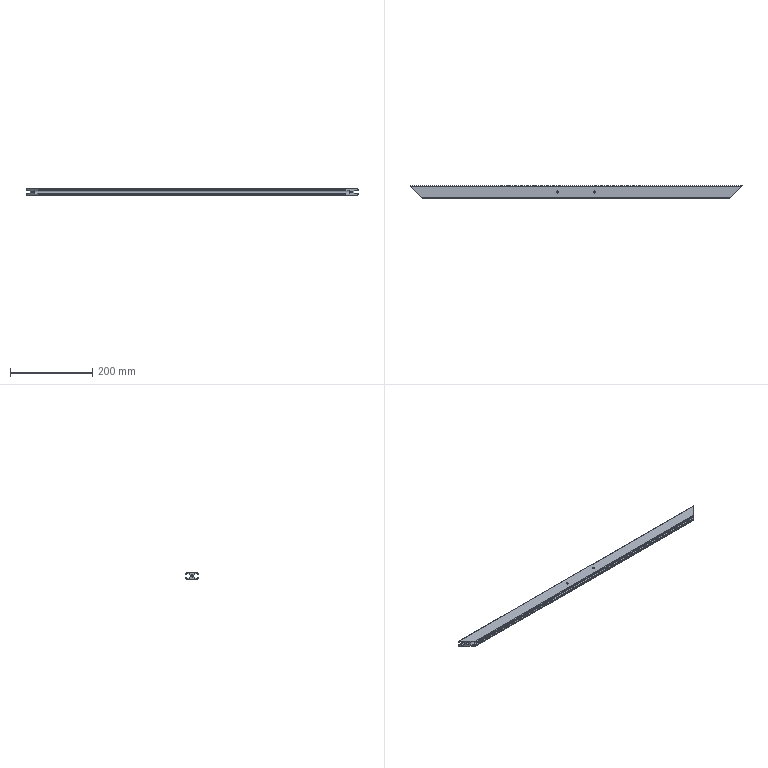Part | SolidWorks | features 3DProfileFeature 1, HoleWzd 1, ICE 1, WeldMemberFeat 1, WeldmentFeature 1 | 1 solid | 40 faces | box 805 x 30 x 15 mm | volume 190827 mm3 | cylinder 20 | plane 20 | commonest cylinder face diameters 5 x14 3 x4 12 x2
STEP:
#1=CARTESIAN_POINT('',(-45.,-2.5,0.));
#2=VERTEX_POINT('',#1);
#3=CARTESIAN_POINT('',(-47.5,0.,2.5));
#4=VERTEX_POINT('',#3);
#5=CARTESIAN_POINT('',(-45.,-2.5,0.));
#6=CARTESIAN_POINT('',(-46.464,-2.5,1.464));
#7=CARTESIAN_POINT('',(-47.5,-1.464,2.5));
#8=CARTESIAN_POINT('',(-47.5,0.,2.5));
#9=(BOUNDED_CURVE()B_SPLINE_CURVE(3,(#5,#6,#7,#8),.UNSPECIFIED.,.F.,.F.)B_SPLINE_CURVE_WITH_KNOTS((4,4),(4.712,6.283),.UNSPECIFIED.)CURVE()GEOMETRIC_REPRESENTATION_ITEM()RATIONAL_B_SPLINE_CURVE((1.,0.8047,0.8047,1.))REPRESENTATION_ITEM(''));
#10=EDGE_CURVE('',#2,#4,#9,.T.);
#11=ORIENTED_EDGE('',*,*,#10,.T.);
#12=CARTESIAN_POINT('',(-47.5,0.,7.5));
#13=VERTEX_POINT('',#12);
#14=CARTESIAN_POINT('',(-47.5,0.,7.5));
#15=DIRECTION('',(0.,0.,1.));
#16=VECTOR('',#15,1000.);
#17=LINE('',#14,#16);
#18=EDGE_CURVE('',#4,#13,#17,.T.);
#19=ORIENTED_EDGE('',*,*,#18,.T.);
#20=CARTESIAN_POINT('',(-42.5,0.,7.5));
#21=VERTEX_POINT('',#20);
#22=CARTESIAN_POINT('',(-45.,0.,7.5));
#23=DIRECTION('',(0.,0.,1.));
#24=DIRECTION('',(1.,0.,0.));
#25=AXIS2_PLACEMENT_3D('',#22,#23,#24);
#26=CIRCLE('',#25,2.5);
#27=EDGE_CURVE('',#13,#21,#26,.T.);
#28=ORIENTED_EDGE('',*,*,#27,.T.);
#29=CARTESIAN_POINT('',(-42.5,0.,2.5));
#30=VERTEX_POINT('',#29);
#31=CARTESIAN_POINT('',(-42.5,0.,7.5));
#32=DIRECTION('',(0.,0.,1.));
#33=VECTOR('',#32,1000.);
#34=LINE('',#31,#33);
#35=EDGE_CURVE('',#30,#21,#34,.T.);
#36=ORIENTED_EDGE('',*,*,#35,.F.);
#37=CARTESIAN_POINT('',(-42.5,0.,2.5));
#38=CARTESIAN_POINT('',(-42.5,-1.464,2.5));
#39=CARTESIAN_POINT('',(-43.536,-2.5,1.464));
#40=CARTESIAN_POINT('',(-45.,-2.5,0.));
#41=(BOUNDED_CURVE()B_SPLINE_CURVE(3,(#37,#38,#39,#40),.UNSPECIFIED.,.F.,.F.)B_SPLINE_CURVE_WITH_KNOTS((4,4),(3.142,4.712),.UNSPECIFIED.)CURVE()GEOMETRIC_REPRESENTATION_ITEM()RATIONAL_B_SPLINE_CURVE((1.,0.8047,0.8047,1.))REPRESENTATION_ITEM(''));
#42=EDGE_CURVE('',#30,#2,#41,.T.);
#43=ORIENTED_EDGE('',*,*,#42,.T.);
#44=EDGE_LOOP('',(#11,#19,#28,#36,#43));
#45=FACE_OUTER_BOUND('',#44,.T.);
#46=CARTESIAN_POINT('',(-45.,0.,7.5));
#47=DIRECTION('',(0.,0.,1.));
#48=DIRECTION('',(1.,0.,0.));
#49=AXIS2_PLACEMENT_3D('',#46,#47,#48);
#50=CYLINDRICAL_SURFACE('',#49,2.5);
#51=ADVANCED_FACE('',(#45),#50,.F.);
#52=CARTESIAN_POINT('',(-47.5,0.,-7.5));
#53=VERTEX_POINT('',#52);
#54=CARTESIAN_POINT('',(-42.5,0.,-7.5));
#55=VERTEX_POINT('',#54);
#56=CARTESIAN_POINT('',(-45.,0.,-7.5));
#57=DIRECTION('',(0.,0.,1.));
#58=DIRECTION('',(1.,0.,0.));
#59=AXIS2_PLACEMENT_3D('',#56,#57,#58);
#60=CIRCLE('',#59,2.5);
#61=EDGE_CURVE('',#53,#55,#60,.T.);
#62=ORIENTED_EDGE('',*,*,#61,.F.);
#63=CARTESIAN_POINT('',(-47.5,0.,-2.5));
#64=VERTEX_POINT('',#63);
#65=CARTESIAN_POINT('',(-47.5,0.,7.5));
#66=DIRECTION('',(0.,0.,1.));
#67=VECTOR('',#66,1000.);
#68=LINE('',#65,#67);
#69=EDGE_CURVE('',#53,#64,#68,.T.);
#70=ORIENTED_EDGE('',*,*,#69,.T.);
#71=CARTESIAN_POINT('',(-47.5,0.,-2.5));
#72=CARTESIAN_POINT('',(-47.5,-1.464,-2.5));
#73=CARTESIAN_POINT('',(-46.464,-2.5,-1.464));
#74=CARTESIAN_POINT('',(-45.,-2.5,0.));
#75=(BOUNDED_CURVE()B_SPLINE_CURVE(3,(#71,#72,#73,#74),.UNSPECIFIED.,.F.,.F.)B_SPLINE_CURVE_WITH_KNOTS((4,4),(0.,1.571),.UNSPECIFIED.)CURVE()GEOMETRIC_REPRESENTATION_ITEM()RATIONAL_B_SPLINE_CURVE((1.,0.8047,0.8047,1.))REPRESENTATION_ITEM(''));
#76=EDGE_CURVE('',#64,#2,#75,.T.);
#77=ORIENTED_EDGE('',*,*,#76,.T.);
#78=CARTESIAN_POINT('',(-42.5,0.,-2.5));
#79=VERTEX_POINT('',#78);
#80=CARTESIAN_POINT('',(-45.,-2.5,0.));
#81=CARTESIAN_POINT('',(-43.536,-2.5,-1.464));
#82=CARTESIAN_POINT('',(-42.5,-1.464,-2.5));
#83=CARTESIAN_POINT('',(-42.5,0.,-2.5));
#84=(BOUNDED_CURVE()B_SPLINE_CURVE(3,(#80,#81,#82,#83),.UNSPECIFIED.,.F.,.F.)B_SPLINE_CURVE_WITH_KNOTS((4,4),(1.571,3.142),.UNSPECIFIED.)CURVE()GEOMETRIC_REPRESENTATION_ITEM()RATIONAL_B_SPLINE_CURVE((1.,0.8047,0.8047,1.))REPRESENTATION_ITEM(''));
#85=EDGE_CURVE('',#2,#79,#84,.T.);
#86=ORIENTED_EDGE('',*,*,#85,.T.);
#87=CARTESIAN_POINT('',(-42.5,0.,7.5));
#88=DIRECTION('',(0.,0.,1.));
#89=VECTOR('',#88,1000.);
#90=LINE('',#87,#89);
#91=EDGE_CURVE('',#55,#79,#90,.T.);
#92=ORIENTED_EDGE('',*,*,#91,.F.);
#93=EDGE_LOOP('',(#62,#70,#77,#86,#92));
#94=FACE_OUTER_BOUND('',#93,.T.);
#95=CARTESIAN_POINT('',(-45.,0.,7.5));
#96=DIRECTION('',(0.,0.,1.));
#97=DIRECTION('',(1.,0.,0.));
#98=AXIS2_PLACEMENT_3D('',#95,#96,#97);
#99=CYLINDRICAL_SURFACE('',#98,2.5);
#100=ADVANCED_FACE('',(#94),#99,.F.);
#101=CARTESIAN_POINT('',(45.,-2.5,0.));
#102=VERTEX_POINT('',#101);
#103=CARTESIAN_POINT('',(42.5,0.,2.5));
#104=VERTEX_POINT('',#103);
#105=CARTESIAN_POINT('',(45.,-2.5,0.));
#106=CARTESIAN_POINT('',(43.536,-2.5,1.464));
#107=CARTESIAN_POINT('',(42.5,-1.464,2.5));
#108=CARTESIAN_POINT('',(42.5,0.,2.5));
#109=(BOUNDED_CURVE()B_SPLINE_CURVE(3,(#105,#106,#107,#108),.UNSPECIFIED.,.F.,.F.)B_SPLINE_CURVE_WITH_KNOTS((4,4),(4.712,6.283),.UNSPECIFIED.)CURVE()GEOMETRIC_REPRESENTATION_ITEM()RATIONAL_B_SPLINE_CURVE((1.,0.8047,0.8047,1.))REPRESENTATION_ITEM(''));
#110=EDGE_CURVE('',#102,#104,#109,.T.);
#111=ORIENTED_EDGE('',*,*,#110,.T.);
#112=CARTESIAN_POINT('',(42.5,0.,7.5));
#113=VERTEX_POINT('',#112);
#114=CARTESIAN_POINT('',(42.5,0.,7.5));
#115=DIRECTION('',(0.,0.,1.));
#116=VECTOR('',#115,1000.);
#117=LINE('',#114,#116);
#118=EDGE_CURVE('',#104,#113,#117,.T.);
#119=ORIENTED_EDGE('',*,*,#118,.T.);
#120=CARTESIAN_POINT('',(47.5,0.,7.5));
#121=VERTEX_POINT('',#120);
#122=CARTESIAN_POINT('',(45.,0.,7.5));
#123=DIRECTION('',(0.,0.,1.));
#124=DIRECTION('',(1.,0.,0.));
#125=AXIS2_PLACEMENT_3D('',#122,#123,#124);
#126=CIRCLE('',#125,2.5);
#127=EDGE_CURVE('',#113,#121,#126,.T.);
#128=ORIENTED_EDGE('',*,*,#127,.T.);
#129=CARTESIAN_POINT('',(47.5,0.,2.5));
#130=VERTEX_POINT('',#129);
#131=CARTESIAN_POINT('',(47.5,0.,7.5));
#132=DIRECTION('',(0.,0.,1.));
#133=VECTOR('',#132,1000.);
#134=LINE('',#131,#133);
#135=EDGE_CURVE('',#130,#121,#134,.T.);
#136=ORIENTED_EDGE('',*,*,#135,.F.);
#137=CARTESIAN_POINT('',(47.5,0.,2.5));
#138=CARTESIAN_POINT('',(47.5,-1.464,2.5));
#139=CARTESIAN_POINT('',(46.464,-2.5,1.464));
#140=CARTESIAN_POINT('',(45.,-2.5,0.));
#141=(BOUNDED_CURVE()B_SPLINE_CURVE(3,(#137,#138,#139,#140),.UNSPECIFIED.,.F.,.F.)B_SPLINE_CURVE_WITH_KNOTS((4,4),(3.142,4.712),.UNSPECIFIED.)CURVE()GEOMETRIC_REPRESENTATION_ITEM()RATIONAL_B_SPLINE_CURVE((1.,0.8047,0.8047,1.))REPRESENTATION_ITEM(''));
#142=EDGE_CURVE('',#130,#102,#141,.T.);
#143=ORIENTED_EDGE('',*,*,#142,.T.);
#144=EDGE_LOOP('',(#111,#119,#128,#136,#143));
#145=FACE_OUTER_BOUND('',#144,.T.);
#146=CARTESIAN_POINT('',(45.,0.,7.5));
#147=DIRECTION('',(0.,0.,1.));
#148=DIRECTION('',(1.,0.,0.));
#149=AXIS2_PLACEMENT_3D('',#146,#147,#148);
#150=CYLINDRICAL_SURFACE('',#149,2.5);
#151=ADVANCED_FACE('',(#145),#150,.F.);
#152=CARTESIAN_POINT('',(42.5,0.,-7.5));
#153=VERTEX_POINT('',#152);
#154=CARTESIAN_POINT('',(47.5,0.,-7.5));
#155=VERTEX_POINT('',#154);
#156=CARTESIAN_POINT('',(45.,0.,-7.5));
#157=DIRECTION('',(0.,0.,1.));
#158=DIRECTION('',(1.,0.,0.));
#159=AXIS2_PLACEMENT_3D('',#156,#157,#158);
#160=CIRCLE('',#159,2.5);
#161=EDGE_CURVE('',#153,#155,#160,.T.);
#162=ORIENTED_EDGE('',*,*,#161,.F.);
#163=CARTESIAN_POINT('',(42.5,0.,-2.5));
#164=VERTEX_POINT('',#163);
#165=CARTESIAN_POINT('',(42.5,0.,7.5));
#166=DIRECTION('',(0.,0.,1.));
#167=VECTOR('',#166,1000.);
#168=LINE('',#165,#167);
#169=EDGE_CURVE('',#153,#164,#168,.T.);
#170=ORIENTED_EDGE('',*,*,#169,.T.);
#171=CARTESIAN_POINT('',(42.5,0.,-2.5));
#172=CARTESIAN_POINT('',(42.5,-1.464,-2.5));
#173=CARTESIAN_POINT('',(43.536,-2.5,-1.464));
#174=CARTESIAN_POINT('',(45.,-2.5,0.));
#175=(BOUNDED_CURVE()B_SPLINE_CURVE(3,(#171,#172,#173,#174),.UNSPECIFIED.,.F.,.F.)B_SPLINE_CURVE_WITH_KNOTS((4,4),(0.,1.571),.UNSPECIFIED.)CURVE()GEOMETRIC_REPRESENTATION_ITEM()RATIONAL_B_SPLINE_CURVE((1.,0.8047,0.8047,1.))REPRESENTATION_ITEM(''));
#176=EDGE_CURVE('',#164,#102,#175,.T.);
#177=ORIENTED_EDGE('',*,*,#176,.T.);
#178=CARTESIAN_POINT('',(47.5,0.,-2.5));
#179=VERTEX_POINT('',#178);
#180=CARTESIAN_POINT('',(45.,-2.5,0.));
#181=CARTESIAN_POINT('',(46.464,-2.5,-1.464));
#182=CARTESIAN_POINT('',(47.5,-1.464,-2.5));
#183=CARTESIAN_POINT('',(47.5,0.,-2.5));
#184=(BOUNDED_CURVE()B_SPLINE_CURVE(3,(#180,#181,#182,#183),.UNSPECIFIED.,.F.,.F.)B_SPLINE_CURVE_WITH_KNOTS((4,4),(1.571,3.142),.UNSPECIFIED.)CURVE()GEOMETRIC_REPRESENTATION_ITEM()RATIONAL_B_SPLINE_CURVE((1.,0.8047,0.8047,1.))REPRESENTATION_ITEM(''));
#185=EDGE_CURVE('',#102,#179,#184,.T.);
#186=ORIENTED_EDGE('',*,*,#185,.T.);
#187=CARTESIAN_POINT('',(47.5,0.,7.5));
#188=DIRECTION('',(0.,0.,1.));
#189=VECTOR('',#188,1000.);
#190=LINE('',#187,#189);
#191=EDGE_CURVE('',#155,#179,#190,.T.);
#192=ORIENTED_EDGE('',*,*,#191,.F.);
#193=EDGE_LOOP('',(#162,#170,#177,#186,#192));
#194=FACE_OUTER_BOUND('',#193,.T.);
#195=CARTESIAN_POINT('',(45.,0.,7.5));
#196=DIRECTION('',(0.,0.,1.));
#197=DIRECTION('',(1.,0.,0.));
#198=AXIS2_PLACEMENT_3D('',#195,#196,#197);
#199=CYLINDRICAL_SURFACE('',#198,2.5);
#200=ADVANCED_FACE('',(#194),#199,.F.);
#201=ORIENTED_EDGE('',*,*,#76,.F.);
#202=CARTESIAN_POINT('',(-387.5,0.,-2.5));
#203=VERTEX_POINT('',#202);
#204=CARTESIAN_POINT('',(402.5,0.,-2.5));
#205=DIRECTION('',(-1.,0.,0.));
#206=VECTOR('',#205,1000.);
#207=LINE('',#204,#206);
#208=EDGE_CURVE('',#64,#203,#207,.T.);
#209=ORIENTED_EDGE('',*,*,#208,.T.);
#210=CARTESIAN_POINT('',(-387.5,0.,2.5));
#211=VERTEX_POINT('',#210);
#212=CARTESIAN_POINT('',(-387.5,0.,2.5));
#213=CARTESIAN_POINT('',(-382.5,-5.,2.5));
#214=CARTESIAN_POINT('',(-382.5,-5.,-2.5));
#215=CARTESIAN_POINT('',(-387.5,0.,-2.5));
#216=(BOUNDED_CURVE()B_SPLINE_CURVE(3,(#212,#213,#214,#215),.UNSPECIFIED.,.F.,.F.)B_SPLINE_CURVE_WITH_KNOTS((4,4),(1.571,4.712),.UNSPECIFIED.)CURVE()GEOMETRIC_REPRESENTATION_ITEM()RATIONAL_B_SPLINE_CURVE((1.,0.3333,0.3333,1.))REPRESENTATION_ITEM(''));
#217=EDGE_CURVE('',#211,#203,#216,.T.);
#218=ORIENTED_EDGE('',*,*,#217,.F.);
#219=CARTESIAN_POINT('',(402.5,0.,2.5));
#220=DIRECTION('',(-1.,0.,0.));
#221=VECTOR('',#220,1000.);
#222=LINE('',#219,#221);
#223=EDGE_CURVE('',#4,#211,#222,.T.);
#224=ORIENTED_EDGE('',*,*,#223,.F.);
#225=ORIENTED_EDGE('',*,*,#10,.F.);
#226=EDGE_LOOP('',(#201,#209,#218,#224,#225));
#227=FACE_OUTER_BOUND('',#226,.T.);
#228=CARTESIAN_POINT('',(402.5,0.,0.));
#229=DIRECTION('',(-1.,0.,0.));
#230=DIRECTION('',(0.,0.,1.));
#231=AXIS2_PLACEMENT_3D('',#228,#229,#230);
#232=CYLINDRICAL_SURFACE('',#231,2.5);
#233=ADVANCED_FACE('',(#227),#232,.F.);
#234=CARTESIAN_POINT('',(387.5,0.,-2.5));
#235=VERTEX_POINT('',#234);
#236=CARTESIAN_POINT('',(387.5,0.,2.5));
#237=VERTEX_POINT('',#236);
#238=CARTESIAN_POINT('',(387.5,0.,-2.5));
#239=CARTESIAN_POINT('',(382.5,-5.,-2.5));
#240=CARTESIAN_POINT('',(382.5,-5.,2.5));
#241=CARTESIAN_POINT('',(387.5,0.,2.5));
#242=(BOUNDED_CURVE()B_SPLINE_CURVE(3,(#238,#239,#240,#241),.UNSPECIFIED.,.F.,.F.)B_SPLINE_CURVE_WITH_KNOTS((4,4),(4.712,7.854),.UNSPECIFIED.)CURVE()GEOMETRIC_REPRESENTATION_ITEM()RATIONAL_B_SPLINE_CURVE((1.,0.3333,0.3333,1.))REPRESENTATION_ITEM(''));
#243=EDGE_CURVE('',#235,#237,#242,.T.);
#244=ORIENTED_EDGE('',*,*,#243,.F.);
#245=CARTESIAN_POINT('',(402.5,0.,-2.5));
#246=DIRECTION('',(-1.,0.,0.));
#247=VECTOR('',#246,1000.);
#248=LINE('',#245,#247);
#249=EDGE_CURVE('',#235,#179,#248,.T.);
#250=ORIENTED_EDGE('',*,*,#249,.T.);
#251=ORIENTED_EDGE('',*,*,#185,.F.);
#252=ORIENTED_EDGE('',*,*,#142,.F.);
#253=CARTESIAN_POINT('',(402.5,0.,2.5));
#254=DIRECTION('',(-1.,0.,0.));
#255=VECTOR('',#254,1000.);
#256=LINE('',#253,#255);
#257=EDGE_CURVE('',#237,#130,#256,.T.);
#258=ORIENTED_EDGE('',*,*,#257,.F.);
#259=EDGE_LOOP('',(#244,#250,#251,#252,#258));
#260=FACE_OUTER_BOUND('',#259,.T.);
#261=CARTESIAN_POINT('',(402.5,0.,0.));
#262=DIRECTION('',(-1.,0.,0.));
#263=DIRECTION('',(0.,0.,1.));
#264=AXIS2_PLACEMENT_3D('',#261,#262,#263);
#265=CYLINDRICAL_SURFACE('',#264,2.5);
#266=ADVANCED_FACE('',(#260),#265,.F.);
#267=ORIENTED_EDGE('',*,*,#176,.F.);
#268=CARTESIAN_POINT('',(402.5,0.,-2.5));
#269=DIRECTION('',(-1.,0.,0.));
#270=VECTOR('',#269,1000.);
#271=LINE('',#268,#270);
#272=EDGE_CURVE('',#164,#79,#271,.T.);
#273=ORIENTED_EDGE('',*,*,#272,.T.);
#274=ORIENTED_EDGE('',*,*,#85,.F.);
#275=ORIENTED_EDGE('',*,*,#42,.F.);
#276=CARTESIAN_POINT('',(402.5,0.,2.5));
#277=DIRECTION('',(-1.,0.,0.));
#278=VECTOR('',#277,1000.);
#279=LINE('',#276,#278);
#280=EDGE_CURVE('',#104,#30,#279,.T.);
#281=ORIENTED_EDGE('',*,*,#280,.F.);
#282=ORIENTED_EDGE('',*,*,#110,.F.);
#283=EDGE_LOOP('',(#267,#273,#274,#275,#281,#282));
#284=FACE_OUTER_BOUND('',#283,.T.);
#285=CARTESIAN_POINT('',(402.5,0.,0.));
#286=DIRECTION('',(-1.,0.,0.));
#287=DIRECTION('',(0.,0.,1.));
#288=AXIS2_PLACEMENT_3D('',#285,#286,#287);
#289=CYLINDRICAL_SURFACE('',#288,2.5);
#290=ADVANCED_FACE('',(#284),#289,.F.);
#291=ORIENTED_EDGE('',*,*,#272,.F.);
#292=CARTESIAN_POINT('',(45.,2.5,0.));
#293=VERTEX_POINT('',#292);
#294=CARTESIAN_POINT('',(45.,2.5,0.));
#295=CARTESIAN_POINT('',(43.536,2.5,-1.464));
#296=CARTESIAN_POINT('',(42.5,1.464,-2.5));
#297=CARTESIAN_POINT('',(42.5,0.,-2.5));
#298=(BOUNDED_CURVE()B_SPLINE_CURVE(3,(#294,#295,#296,#297),.UNSPECIFIED.,.F.,.F.)B_SPLINE_CURVE_WITH_KNOTS((4,4),(4.712,6.283),.UNSPECIFIED.)CURVE()GEOMETRIC_REPRESENTATION_ITEM()RATIONAL_B_SPLINE_CURVE((1.,0.8047,0.8047,1.))REPRESENTATION_ITEM(''));
#299=EDGE_CURVE('',#293,#164,#298,.T.);
#300=ORIENTED_EDGE('',*,*,#299,.F.);
#301=CARTESIAN_POINT('',(42.5,0.,2.5));
#302=CARTESIAN_POINT('',(42.5,1.464,2.5));
#303=CARTESIAN_POINT('',(43.536,2.5,1.464));
#304=CARTESIAN_POINT('',(45.,2.5,0.));
#305=(BOUNDED_CURVE()B_SPLINE_CURVE(3,(#301,#302,#303,#304),.UNSPECIFIED.,.F.,.T.)B_SPLINE_CURVE_WITH_KNOTS((4,4),(0.,1.571),.UNSPECIFIED.)CURVE()GEOMETRIC_REPRESENTATION_ITEM()RATIONAL_B_SPLINE_CURVE((1.,0.8047,0.8047,1.))REPRESENTATION_ITEM(''));
#306=EDGE_CURVE('',#104,#293,#305,.T.);
#307=ORIENTED_EDGE('',*,*,#306,.F.);
#308=ORIENTED_EDGE('',*,*,#280,.T.);
#309=CARTESIAN_POINT('',(-45.,2.5,0.));
#310=VERTEX_POINT('',#309);
#311=CARTESIAN_POINT('',(-45.,2.5,0.));
#312=CARTESIAN_POINT('',(-43.536,2.5,1.464));
#313=CARTESIAN_POINT('',(-42.5,1.464,2.5));
#314=CARTESIAN_POINT('',(-42.5,0.,2.5));
#315=(BOUNDED_CURVE()B_SPLINE_CURVE(3,(#311,#312,#313,#314),.UNSPECIFIED.,.F.,.F.)B_SPLINE_CURVE_WITH_KNOTS((4,4),(1.571,3.142),.UNSPECIFIED.)CURVE()GEOMETRIC_REPRESENTATION_ITEM()RATIONAL_B_SPLINE_CURVE((1.,0.8047,0.8047,1.))REPRESENTATION_ITEM(''));
#316=EDGE_CURVE('',#310,#30,#315,.T.);
#317=ORIENTED_EDGE('',*,*,#316,.F.);
#318=CARTESIAN_POINT('',(-42.5,0.,-2.5));
#319=CARTESIAN_POINT('',(-42.5,1.464,-2.5));
#320=CARTESIAN_POINT('',(-43.536,2.5,-1.464));
#321=CARTESIAN_POINT('',(-45.,2.5,0.));
#322=(BOUNDED_CURVE()B_SPLINE_CURVE(3,(#318,#319,#320,#321),.UNSPECIFIED.,.F.,.F.)B_SPLINE_CURVE_WITH_KNOTS((4,4),(3.142,4.712),.UNSPECIFIED.)CURVE()GEOMETRIC_REPRESENTATION_ITEM()RATIONAL_B_SPLINE_CURVE((1.,0.8047,0.8047,1.))REPRESENTATION_ITEM(''));
#323=EDGE_CURVE('',#79,#310,#322,.T.);
#324=ORIENTED_EDGE('',*,*,#323,.F.);
#325=EDGE_LOOP('',(#291,#300,#307,#308,#317,#324));
#326=FACE_OUTER_BOUND('',#325,.T.);
#327=CARTESIAN_POINT('',(402.5,0.,0.));
#328=DIRECTION('',(-1.,0.,0.));
#329=DIRECTION('',(0.,0.,1.));
#330=AXIS2_PLACEMENT_3D('',#327,#328,#329);
#331=CYLINDRICAL_SURFACE('',#330,2.5);
#332=ADVANCED_FACE('',(#326),#331,.F.);
#333=ORIENTED_EDGE('',*,*,#249,.F.);
#334=CARTESIAN_POINT('',(387.5,0.,2.5));
#335=CARTESIAN_POINT('',(392.5,5.,2.5));
#336=CARTESIAN_POINT('',(392.5,5.,-2.5));
#337=CARTESIAN_POINT('',(387.5,0.,-2.5));
#338=(BOUNDED_CURVE()B_SPLINE_CURVE(3,(#334,#335,#336,#337),.UNSPECIFIED.,.F.,.F.)B_SPLINE_CURVE_WITH_KNOTS((4,4),(1.571,4.712),.UNSPECIFIED.)CURVE()GEOMETRIC_REPRESENTATION_ITEM()RATIONAL_B_SPLINE_CURVE((1.,0.3333,0.3333,1.))REPRESENTATION_ITEM(''));
#339=EDGE_CURVE('',#237,#235,#338,.T.);
#340=ORIENTED_EDGE('',*,*,#339,.F.);
#341=ORIENTED_EDGE('',*,*,#257,.T.);
#342=CARTESIAN_POINT('',(45.,2.5,0.));
#343=CARTESIAN_POINT('',(46.464,2.5,1.464));
#344=CARTESIAN_POINT('',(47.5,1.464,2.5));
#345=CARTESIAN_POINT('',(47.5,0.,2.5));
#346=(BOUNDED_CURVE()B_SPLINE_CURVE(3,(#342,#343,#344,#345),.UNSPECIFIED.,.F.,.F.)B_SPLINE_CURVE_WITH_KNOTS((4,4),(1.571,3.142),.UNSPECIFIED.)CURVE()GEOMETRIC_REPRESENTATION_ITEM()RATIONAL_B_SPLINE_CURVE((1.,0.8047,0.8047,1.))REPRESENTATION_ITEM(''));
#347=EDGE_CURVE('',#293,#130,#346,.T.);
#348=ORIENTED_EDGE('',*,*,#347,.F.);
#349=CARTESIAN_POINT('',(47.5,0.,-2.5));
#350=CARTESIAN_POINT('',(47.5,1.464,-2.5));
#351=CARTESIAN_POINT('',(46.464,2.5,-1.464));
#352=CARTESIAN_POINT('',(45.,2.5,0.));
#353=(BOUNDED_CURVE()B_SPLINE_CURVE(3,(#349,#350,#351,#352),.UNSPECIFIED.,.F.,.F.)B_SPLINE_CURVE_WITH_KNOTS((4,4),(3.142,4.712),.UNSPECIFIED.)CURVE()GEOMETRIC_REPRESENTATION_ITEM()RATIONAL_B_SPLINE_CURVE((1.,0.8047,0.8047,1.))REPRESENTATION_ITEM(''));
#354=EDGE_CURVE('',#179,#293,#353,.T.);
#355=ORIENTED_EDGE('',*,*,#354,.F.);
#356=EDGE_LOOP('',(#333,#340,#341,#348,#355));
#357=FACE_OUTER_BOUND('',#356,.T.);
#358=CARTESIAN_POINT('',(402.5,0.,0.));
#359=DIRECTION('',(-1.,0.,0.));
#360=DIRECTION('',(0.,0.,1.));
#361=AXIS2_PLACEMENT_3D('',#358,#359,#360);
#362=CYLINDRICAL_SURFACE('',#361,2.5);
#363=ADVANCED_FACE('',(#357),#362,.F.);
#364=CARTESIAN_POINT('',(402.5,15.,3.25));
#365=VERTEX_POINT('',#364);
#366=CARTESIAN_POINT('',(-402.5,15.,3.25));
#367=VERTEX_POINT('',#366);
#368=CARTESIAN_POINT('',(402.5,15.,3.25));
#369=DIRECTION('',(-1.,0.,0.));
#370=VECTOR('',#369,1000.);
#371=LINE('',#368,#370);
#372=EDGE_CURVE('',#365,#367,#371,.T.);
#373=ORIENTED_EDGE('',*,*,#372,.F.);
#374=CARTESIAN_POINT('',(400.2,12.7,3.25));
#375=VERTEX_POINT('',#374);
#376=CARTESIAN_POINT('',(402.5,15.,3.25));
#377=DIRECTION('',(-0.7071,-0.7071,0.));
#378=VECTOR('',#377,1000.);
#379=LINE('',#376,#378);
#380=EDGE_CURVE('',#365,#375,#379,.T.);
#381=ORIENTED_EDGE('',*,*,#380,.T.);
#382=CARTESIAN_POINT('',(-400.2,12.7,3.25));
#383=VERTEX_POINT('',#382);
#384=CARTESIAN_POINT('',(402.5,12.7,3.25));
#385=DIRECTION('',(-1.,0.,0.));
#386=VECTOR('',#385,1000.);
#387=LINE('',#384,#386);
#388=EDGE_CURVE('',#375,#383,#387,.T.);
#389=ORIENTED_EDGE('',*,*,#388,.T.);
#390=CARTESIAN_POINT('',(0.,-387.5,3.25));
#391=DIRECTION('',(-0.7071,0.7071,0.));
#392=VECTOR('',#391,1000.);
#393=LINE('',#390,#392);
#394=EDGE_CURVE('',#383,#367,#393,.T.);
#395=ORIENTED_EDGE('',*,*,#394,.T.);
#396=EDGE_LOOP('',(#373,#381,#389,#395));
#397=FACE_OUTER_BOUND('',#396,.T.);
#398=CARTESIAN_POINT('',(402.5,15.,3.25));
#399=DIRECTION('',(0.,0.,1.));
#400=DIRECTION('',(0.,-1.,0.));
#401=AXIS2_PLACEMENT_3D('',#398,#399,#400);
#402=PLANE('',#401);
#403=ADVANCED_FACE('',(#397),#402,.F.);
#404=CARTESIAN_POINT('',(-402.5,15.,6.));
#405=VERTEX_POINT('',#404);
#406=CARTESIAN_POINT('',(-402.5,15.,6.));
#407=DIRECTION('',(0.,0.,1.));
#408=VECTOR('',#407,1000.);
#409=LINE('',#406,#408);
#410=EDGE_CURVE('',#367,#405,#409,.T.);
#411=ORIENTED_EDGE('',*,*,#410,.T.);
#412=CARTESIAN_POINT('',(402.5,15.,6.));
#413=VERTEX_POINT('',#412);
#414=CARTESIAN_POINT('',(402.5,15.,6.));
#415=DIRECTION('',(-1.,0.,0.));
#416=VECTOR('',#415,1000.);
#417=LINE('',#414,#416);
#418=EDGE_CURVE('',#413,#405,#417,.T.);
#419=ORIENTED_EDGE('',*,*,#418,.F.);
#420=CARTESIAN_POINT('',(402.5,15.,6.));
#421=DIRECTION('',(0.,0.,1.));
#422=VECTOR('',#421,1000.);
#423=LINE('',#420,#422);
#424=EDGE_CURVE('',#365,#413,#423,.T.);
#425=ORIENTED_EDGE('',*,*,#424,.F.);
#426=ORIENTED_EDGE('',*,*,#372,.T.);
#427=EDGE_LOOP('',(#411,#419,#425,#426));
#428=FACE_OUTER_BOUND('',#427,.T.);
#429=CARTESIAN_POINT('',(402.5,15.,6.));
#430=DIRECTION('',(0.,-1.,0.));
#431=DIRECTION('',(0.,0.,-1.));
#432=AXIS2_PLACEMENT_3D('',#429,#430,#431);
#433=PLANE('',#432);
#434=ADVANCED_FACE('',(#428),#433,.F.);
#435=CARTESIAN_POINT('',(401.,13.5,7.5));
#436=VERTEX_POINT('',#435);
#437=CARTESIAN_POINT('',(-401.,13.5,7.5));
#438=VERTEX_POINT('',#437);
#439=CARTESIAN_POINT('',(402.5,13.5,7.5));
#440=DIRECTION('',(-1.,0.,0.));
#441=VECTOR('',#440,1000.);
#442=LINE('',#439,#441);
#443=EDGE_CURVE('',#436,#438,#442,.T.);
#444=ORIENTED_EDGE('',*,*,#443,.F.);
#445=CARTESIAN_POINT('',(401.,13.5,7.5));
#446=CARTESIAN_POINT('',(401.879,14.379,7.5));
#447=CARTESIAN_POINT('',(402.5,15.,6.879));
#448=CARTESIAN_POINT('',(402.5,15.,6.));
#449=(BOUNDED_CURVE()B_SPLINE_CURVE(3,(#445,#446,#447,#448),.UNSPECIFIED.,.F.,.F.)B_SPLINE_CURVE_WITH_KNOTS((4,4),(1.571,3.142),.UNSPECIFIED.)CURVE()GEOMETRIC_REPRESENTATION_ITEM()RATIONAL_B_SPLINE_CURVE((1.,0.8047,0.8047,1.))REPRESENTATION_ITEM(''));
#450=EDGE_CURVE('',#436,#413,#449,.T.);
#451=ORIENTED_EDGE('',*,*,#450,.T.);
#452=ORIENTED_EDGE('',*,*,#418,.T.);
#453=CARTESIAN_POINT('',(-402.5,15.,6.));
#454=CARTESIAN_POINT('',(-402.5,15.,6.879));
#455=CARTESIAN_POINT('',(-401.879,14.379,7.5));
#456=CARTESIAN_POINT('',(-401.,13.5,7.5));
#457=(BOUNDED_CURVE()B_SPLINE_CURVE(3,(#453,#454,#455,#456),.UNSPECIFIED.,.F.,.F.)B_SPLINE_CURVE_WITH_KNOTS((4,4),(0.,1.571),.UNSPECIFIED.)CURVE()GEOMETRIC_REPRESENTATION_ITEM()RATIONAL_B_SPLINE_CURVE((1.,0.8047,0.8047,1.))REPRESENTATION_ITEM(''));
#458=EDGE_CURVE('',#405,#438,#457,.T.);
#459=ORIENTED_EDGE('',*,*,#458,.T.);
#460=EDGE_LOOP('',(#444,#451,#452,#459));
#461=FACE_OUTER_BOUND('',#460,.T.);
#462=CARTESIAN_POINT('',(402.5,13.5,6.));
#463=DIRECTION('',(-1.,0.,0.));
#464=DIRECTION('',(0.,0.,1.));
#465=AXIS2_PLACEMENT_3D('',#462,#463,#464);
#466=CYLINDRICAL_SURFACE('',#465,1.5);
#467=ADVANCED_FACE('',(#461),#466,.T.);
#468=CARTESIAN_POINT('',(-45.,0.,7.5));
#469=DIRECTION('',(0.,0.,1.));
#470=DIRECTION('',(1.,0.,0.));
#471=AXIS2_PLACEMENT_3D('',#468,#469,#470);
#472=CIRCLE('',#471,2.5);
#473=EDGE_CURVE('',#21,#13,#472,.T.);
#474=ORIENTED_EDGE('',*,*,#473,.F.);
#475=ORIENTED_EDGE('',*,*,#27,.F.);
#476=EDGE_LOOP('',(#474,#475));
#477=FACE_BOUND('',#476,.T.);
#478=CARTESIAN_POINT('',(45.,0.,7.5));
#479=DIRECTION('',(0.,0.,1.));
#480=DIRECTION('',(1.,0.,0.));
#481=AXIS2_PLACEMENT_3D('',#478,#479,#480);
#482=CIRCLE('',#481,2.5);
#483=EDGE_CURVE('',#121,#113,#482,.T.);
#484=ORIENTED_EDGE('',*,*,#483,.F.);
#485=ORIENTED_EDGE('',*,*,#127,.F.);
#486=EDGE_LOOP('',(#484,#485));
#487=FACE_BOUND('',#486,.T.);
#488=CARTESIAN_POINT('',(374.,-13.5,7.5));
#489=VERTEX_POINT('',#488);
#490=CARTESIAN_POINT('',(-374.,-13.5,7.5));
#491=VERTEX_POINT('',#490);
#492=CARTESIAN_POINT('',(402.5,-13.5,7.5));
#493=DIRECTION('',(-1.,0.,0.));
#494=VECTOR('',#493,1000.);
#495=LINE('',#492,#494);
#496=EDGE_CURVE('',#489,#491,#495,.T.);
#497=ORIENTED_EDGE('',*,*,#496,.F.);
#498=CARTESIAN_POINT('',(402.5,15.,7.5));
#499=DIRECTION('',(-0.7071,-0.7071,0.));
#500=VECTOR('',#499,1000.);
#501=LINE('',#498,#500);
#502=EDGE_CURVE('',#436,#489,#501,.T.);
#503=ORIENTED_EDGE('',*,*,#502,.F.);
#504=ORIENTED_EDGE('',*,*,#443,.T.);
#505=CARTESIAN_POINT('',(-402.5,15.,7.5));
#506=DIRECTION('',(-0.7071,0.7071,0.));
#507=VECTOR('',#506,1000.);
#508=LINE('',#505,#507);
#509=EDGE_CURVE('',#491,#438,#508,.T.);
#510=ORIENTED_EDGE('',*,*,#509,.F.);
#511=EDGE_LOOP('',(#497,#503,#504,#510));
#512=FACE_OUTER_BOUND('',#511,.T.);
#513=CARTESIAN_POINT('',(402.5,-13.5,7.5));
#514=DIRECTION('',(0.,0.,-1.));
#515=DIRECTION('',(-1.,0.,0.));
#516=AXIS2_PLACEMENT_3D('',#513,#514,#515);
#517=PLANE('',#516);
#518=ADVANCED_FACE('',(#477,#487,#512),#517,.F.);
#519=CARTESIAN_POINT('',(372.5,-15.,6.));
#520=VERTEX_POINT('',#519);
#521=CARTESIAN_POINT('',(-372.5,-15.,6.));
#522=VERTEX_POINT('',#521);
#523=CARTESIAN_POINT('',(402.5,-15.,6.));
#524=DIRECTION('',(-1.,0.,0.));
#525=VECTOR('',#524,1000.);
#526=LINE('',#523,#525);
#527=EDGE_CURVE('',#520,#522,#526,.T.);
#528=ORIENTED_EDGE('',*,*,#527,.F.);
#529=CARTESIAN_POINT('',(372.5,-15.,6.));
#530=CARTESIAN_POINT('',(372.5,-15.,6.879));
#531=CARTESIAN_POINT('',(373.121,-14.379,7.5));
#532=CARTESIAN_POINT('',(374.,-13.5,7.5));
#533=(BOUNDED_CURVE()B_SPLINE_CURVE(3,(#529,#530,#531,#532),.UNSPECIFIED.,.F.,.F.)B_SPLINE_CURVE_WITH_KNOTS((4,4),(0.,1.571),.UNSPECIFIED.)CURVE()GEOMETRIC_REPRESENTATION_ITEM()RATIONAL_B_SPLINE_CURVE((1.,0.8047,0.8047,1.))REPRESENTATION_ITEM(''));
#534=EDGE_CURVE('',#520,#489,#533,.T.);
#535=ORIENTED_EDGE('',*,*,#534,.T.);
#536=ORIENTED_EDGE('',*,*,#496,.T.);
#537=CARTESIAN_POINT('',(-374.,-13.5,7.5));
#538=CARTESIAN_POINT('',(-373.121,-14.379,7.5));
#539=CARTESIAN_POINT('',(-372.5,-15.,6.879));
#540=CARTESIAN_POINT('',(-372.5,-15.,6.));
#541=(BOUNDED_CURVE()B_SPLINE_CURVE(3,(#537,#538,#539,#540),.UNSPECIFIED.,.F.,.F.)B_SPLINE_CURVE_WITH_KNOTS((4,4),(1.571,3.142),.UNSPECIFIED.)CURVE()GEOMETRIC_REPRESENTATION_ITEM()RATIONAL_B_SPLINE_CURVE((1.,0.8047,0.8047,1.))REPRESENTATION_ITEM(''));
#542=EDGE_CURVE('',#491,#522,#541,.T.);
#543=ORIENTED_EDGE('',*,*,#542,.T.);
#544=EDGE_LOOP('',(#528,#535,#536,#543));
#545=FACE_OUTER_BOUND('',#544,.T.);
#546=CARTESIAN_POINT('',(402.5,-13.5,6.));
#547=DIRECTION('',(-1.,0.,0.));
#548=DIRECTION('',(0.,0.,1.));
#549=AXIS2_PLACEMENT_3D('',#546,#547,#548);
#550=CYLINDRICAL_SURFACE('',#549,1.5);
#551=ADVANCED_FACE('',(#545),#550,.T.);
#552=CARTESIAN_POINT('',(372.5,-15.,3.25));
#553=VERTEX_POINT('',#552);
#554=CARTESIAN_POINT('',(-372.5,-15.,3.25));
#555=VERTEX_POINT('',#554);
#556=CARTESIAN_POINT('',(402.5,-15.,3.25));
#557=DIRECTION('',(-1.,0.,0.));
#558=VECTOR('',#557,1000.);
#559=LINE('',#556,#558);
#560=EDGE_CURVE('',#553,#555,#559,.T.);
#561=ORIENTED_EDGE('',*,*,#560,.F.);
#562=CARTESIAN_POINT('',(372.5,-15.,-7.5));
#563=DIRECTION('',(0.,0.,1.));
#564=VECTOR('',#563,1000.);
#565=LINE('',#562,#564);
#566=EDGE_CURVE('',#553,#520,#565,.T.);
#567=ORIENTED_EDGE('',*,*,#566,.T.);
#568=ORIENTED_EDGE('',*,*,#527,.T.);
#569=CARTESIAN_POINT('',(-372.5,-15.,-7.5));
#570=DIRECTION('',(0.,0.,1.));
#571=VECTOR('',#570,1000.);
#572=LINE('',#569,#571);
#573=EDGE_CURVE('',#555,#522,#572,.T.);
#574=ORIENTED_EDGE('',*,*,#573,.F.);
#575=EDGE_LOOP('',(#561,#567,#568,#574));
#576=FACE_OUTER_BOUND('',#575,.T.);
#577=CARTESIAN_POINT('',(402.5,-15.,6.));
#578=DIRECTION('',(0.,1.,0.));
#579=DIRECTION('',(0.,0.,1.));
#580=AXIS2_PLACEMENT_3D('',#577,#578,#579);
#581=PLANE('',#580);
#582=ADVANCED_FACE('',(#576),#581,.F.);
#583=CARTESIAN_POINT('',(374.8,-12.7,3.25));
#584=VERTEX_POINT('',#583);
#585=CARTESIAN_POINT('',(-374.8,-12.7,3.25));
#586=VERTEX_POINT('',#585);
#587=CARTESIAN_POINT('',(402.5,-12.7,3.25));
#588=DIRECTION('',(-1.,0.,0.));
#589=VECTOR('',#588,1000.);
#590=LINE('',#587,#589);
#591=EDGE_CURVE('',#584,#586,#590,.T.);
#592=ORIENTED_EDGE('',*,*,#591,.F.);
#593=CARTESIAN_POINT('',(387.5,0.,3.25));
#594=DIRECTION('',(-0.7071,-0.7071,0.));
#595=VECTOR('',#594,1000.);
#596=LINE('',#593,#595);
#597=EDGE_CURVE('',#584,#553,#596,.T.);
#598=ORIENTED_EDGE('',*,*,#597,.T.);
#599=ORIENTED_EDGE('',*,*,#560,.T.);
#600=CARTESIAN_POINT('',(15.,-402.5,3.25));
#601=DIRECTION('',(-0.7071,0.7071,0.));
#602=VECTOR('',#601,1000.);
#603=LINE('',#600,#602);
#604=EDGE_CURVE('',#555,#586,#603,.T.);
#605=ORIENTED_EDGE('',*,*,#604,.T.);
#606=EDGE_LOOP('',(#592,#598,#599,#605));
#607=FACE_OUTER_BOUND('',#606,.T.);
#608=CARTESIAN_POINT('',(402.5,-15.,3.25));
#609=DIRECTION('',(0.,0.,1.));
#610=DIRECTION('',(0.,-1.,0.));
#611=AXIS2_PLACEMENT_3D('',#608,#609,#610);
#612=PLANE('',#611);
#613=ADVANCED_FACE('',(#607),#612,.F.);
#614=CARTESIAN_POINT('',(374.8,-12.7,5.));
#615=VERTEX_POINT('',#614);
#616=CARTESIAN_POINT('',(-374.8,-12.7,5.));
#617=VERTEX_POINT('',#616);
#618=CARTESIAN_POINT('',(402.5,-12.7,5.));
#619=DIRECTION('',(-1.,0.,0.));
#620=VECTOR('',#619,1000.);
#621=LINE('',#618,#620);
#622=EDGE_CURVE('',#615,#617,#621,.T.);
#623=ORIENTED_EDGE('',*,*,#622,.F.);
#624=CARTESIAN_POINT('',(374.8,-12.7,3.25));
#625=DIRECTION('',(0.,0.,-1.));
#626=VECTOR('',#625,1000.);
#627=LINE('',#624,#626);
#628=EDGE_CURVE('',#615,#584,#627,.T.);
#629=ORIENTED_EDGE('',*,*,#628,.T.);
#630=ORIENTED_EDGE('',*,*,#591,.T.);
#631=CARTESIAN_POINT('',(-374.8,-12.7,3.25));
#632=DIRECTION('',(0.,0.,1.));
#633=VECTOR('',#632,1000.);
#634=LINE('',#631,#633);
#635=EDGE_CURVE('',#586,#617,#634,.T.);
#636=ORIENTED_EDGE('',*,*,#635,.T.);
#637=EDGE_LOOP('',(#623,#629,#630,#636));
#638=FACE_OUTER_BOUND('',#637,.T.);
#639=CARTESIAN_POINT('',(402.5,-12.7,3.25));
#640=DIRECTION('',(0.,-1.,0.));
#641=DIRECTION('',(0.,0.,-1.));
#642=AXIS2_PLACEMENT_3D('',#639,#640,#641);
#643=PLANE('',#642);
#644=ADVANCED_FACE('',(#638),#643,.F.);
#645=CARTESIAN_POINT('',(380.5,-7.,5.));
#646=VERTEX_POINT('',#645);
#647=CARTESIAN_POINT('',(-380.5,-7.,5.));
#648=VERTEX_POINT('',#647);
#649=CARTESIAN_POINT('',(402.5,-7.,5.));
#650=DIRECTION('',(-1.,0.,0.));
#651=VECTOR('',#650,1000.);
#652=LINE('',#649,#651);
#653=EDGE_CURVE('',#646,#648,#652,.T.);
#654=ORIENTED_EDGE('',*,*,#653,.F.);
#655=CARTESIAN_POINT('',(388.65,1.15,5.));
#656=DIRECTION('',(-0.7071,-0.7071,0.));
#657=VECTOR('',#656,1000.);
#658=LINE('',#655,#657);
#659=EDGE_CURVE('',#646,#615,#658,.T.);
#660=ORIENTED_EDGE('',*,*,#659,.T.);
#661=ORIENTED_EDGE('',*,*,#622,.T.);
#662=CARTESIAN_POINT('',(13.85,-401.35,5.));
#663=DIRECTION('',(-0.7071,0.7071,0.));
#664=VECTOR('',#663,1000.);
#665=LINE('',#662,#664);
#666=EDGE_CURVE('',#617,#648,#665,.T.);
#667=ORIENTED_EDGE('',*,*,#666,.T.);
#668=EDGE_LOOP('',(#654,#660,#661,#667));
#669=FACE_OUTER_BOUND('',#668,.T.);
#670=CARTESIAN_POINT('',(402.5,-12.7,5.));
#671=DIRECTION('',(0.,0.,1.));
#672=DIRECTION('',(0.,-1.,0.));
#673=AXIS2_PLACEMENT_3D('',#670,#671,#672);
#674=PLANE('',#673);
#675=ADVANCED_FACE('',(#669),#674,.F.);
#676=CARTESIAN_POINT('',(380.5,-7.,-5.));
#677=VERTEX_POINT('',#676);
#678=CARTESIAN_POINT('',(-380.5,-7.,-5.));
#679=VERTEX_POINT('',#678);
#680=CARTESIAN_POINT('',(402.5,-7.,-5.));
#681=DIRECTION('',(-1.,0.,0.));
#682=VECTOR('',#681,1000.);
#683=LINE('',#680,#682);
#684=EDGE_CURVE('',#677,#679,#683,.T.);
#685=ORIENTED_EDGE('',*,*,#684,.F.);
#686=CARTESIAN_POINT('',(380.5,-7.,-5.));
#687=CARTESIAN_POINT('',(384.458,-3.042,-2.375));
#688=CARTESIAN_POINT('',(384.458,-3.042,2.375));
#689=CARTESIAN_POINT('',(380.5,-7.,5.));
#690=(BOUNDED_CURVE()B_SPLINE_CURVE(3,(#686,#687,#688,#689),.UNSPECIFIED.,.F.,.F.)B_SPLINE_CURVE_WITH_KNOTS((4,4),(2.156,4.127),.UNSPECIFIED.)CURVE()GEOMETRIC_REPRESENTATION_ITEM()RATIONAL_B_SPLINE_CURVE((1.,0.7018,0.7018,1.))REPRESENTATION_ITEM(''));
#691=EDGE_CURVE('',#677,#646,#690,.T.);
#692=ORIENTED_EDGE('',*,*,#691,.T.);
#693=ORIENTED_EDGE('',*,*,#653,.T.);
#694=CARTESIAN_POINT('',(-380.5,-7.,5.));
#695=CARTESIAN_POINT('',(-384.458,-3.042,2.375));
#696=CARTESIAN_POINT('',(-384.458,-3.042,-2.375));
#697=CARTESIAN_POINT('',(-380.5,-7.,-5.));
#698=(BOUNDED_CURVE()B_SPLINE_CURVE(3,(#694,#695,#696,#697),.UNSPECIFIED.,.F.,.F.)B_SPLINE_CURVE_WITH_KNOTS((4,4),(5.298,7.268),.UNSPECIFIED.)CURVE()GEOMETRIC_REPRESENTATION_ITEM()RATIONAL_B_SPLINE_CURVE((1.,0.7018,0.7018,1.))REPRESENTATION_ITEM(''));
#699=EDGE_CURVE('',#648,#679,#698,.T.);
#700=ORIENTED_EDGE('',*,*,#699,.T.);
#701=EDGE_LOOP('',(#685,#692,#693,#700));
#702=FACE_OUTER_BOUND('',#701,.T.);
#703=CARTESIAN_POINT('',(402.5,-10.317,0.));
#704=DIRECTION('',(-1.,0.,0.));
#705=DIRECTION('',(0.,0.,1.));
#706=AXIS2_PLACEMENT_3D('',#703,#704,#705);
#707=CYLINDRICAL_SURFACE('',#706,6.);
#708=ADVANCED_FACE('',(#702),#707,.F.);
#709=CARTESIAN_POINT('',(374.8,-12.7,-5.));
#710=VERTEX_POINT('',#709);
#711=CARTESIAN_POINT('',(-374.8,-12.7,-5.));
#712=VERTEX_POINT('',#711);
#713=CARTESIAN_POINT('',(402.5,-12.7,-5.));
#714=DIRECTION('',(-1.,0.,0.));
#715=VECTOR('',#714,1000.);
#716=LINE('',#713,#715);
#717=EDGE_CURVE('',#710,#712,#716,.T.);
#718=ORIENTED_EDGE('',*,*,#717,.F.);
#719=CARTESIAN_POINT('',(388.65,1.15,-5.));
#720=DIRECTION('',(0.7071,0.7071,0.));
#721=VECTOR('',#720,1000.);
#722=LINE('',#719,#721);
#723=EDGE_CURVE('',#710,#677,#722,.T.);
#724=ORIENTED_EDGE('',*,*,#723,.T.);
#725=ORIENTED_EDGE('',*,*,#684,.T.);
#726=CARTESIAN_POINT('',(13.85,-401.35,-5.));
#727=DIRECTION('',(0.7071,-0.7071,0.));
#728=VECTOR('',#727,1000.);
#729=LINE('',#726,#728);
#730=EDGE_CURVE('',#679,#712,#729,.T.);
#731=ORIENTED_EDGE('',*,*,#730,.T.);
#732=EDGE_LOOP('',(#718,#724,#725,#731));
#733=FACE_OUTER_BOUND('',#732,.T.);
#734=CARTESIAN_POINT('',(402.5,-12.7,-5.));
#735=DIRECTION('',(0.,0.,-1.));
#736=DIRECTION('',(0.,1.,0.));
#737=AXIS2_PLACEMENT_3D('',#734,#735,#736);
#738=PLANE('',#737);
#739=ADVANCED_FACE('',(#733),#738,.F.);
#740=CARTESIAN_POINT('',(374.8,-12.7,-3.25));
#741=VERTEX_POINT('',#740);
#742=CARTESIAN_POINT('',(-374.8,-12.7,-3.25));
#743=VERTEX_POINT('',#742);
#744=CARTESIAN_POINT('',(402.5,-12.7,-3.25));
#745=DIRECTION('',(-1.,0.,0.));
#746=VECTOR('',#745,1000.);
#747=LINE('',#744,#746);
#748=EDGE_CURVE('',#741,#743,#747,.T.);
#749=ORIENTED_EDGE('',*,*,#748,.F.);
#750=CARTESIAN_POINT('',(374.8,-12.7,-3.25));
#751=DIRECTION('',(0.,0.,-1.));
#752=VECTOR('',#751,1000.);
#753=LINE('',#750,#752);
#754=EDGE_CURVE('',#741,#710,#753,.T.);
#755=ORIENTED_EDGE('',*,*,#754,.T.);
#756=ORIENTED_EDGE('',*,*,#717,.T.);
#757=CARTESIAN_POINT('',(-374.8,-12.7,-3.25));
#758=DIRECTION('',(0.,0.,1.));
#759=VECTOR('',#758,1000.);
#760=LINE('',#757,#759);
#761=EDGE_CURVE('',#712,#743,#760,.T.);
#762=ORIENTED_EDGE('',*,*,#761,.T.);
#763=EDGE_LOOP('',(#749,#755,#756,#762));
#764=FACE_OUTER_BOUND('',#763,.T.);
#765=CARTESIAN_POINT('',(402.5,-12.7,-3.25));
#766=DIRECTION('',(0.,-1.,0.));
#767=DIRECTION('',(0.,0.,-1.));
#768=AXIS2_PLACEMENT_3D('',#765,#766,#767);
#769=PLANE('',#768);
#770=ADVANCED_FACE('',(#764),#769,.F.);
#771=CARTESIAN_POINT('',(372.5,-15.,-3.25));
#772=VERTEX_POINT('',#771);
#773=CARTESIAN_POINT('',(-372.5,-15.,-3.25));
#774=VERTEX_POINT('',#773);
#775=CARTESIAN_POINT('',(402.5,-15.,-3.25));
#776=DIRECTION('',(-1.,0.,0.));
#777=VECTOR('',#776,1000.);
#778=LINE('',#775,#777);
#779=EDGE_CURVE('',#772,#774,#778,.T.);
#780=ORIENTED_EDGE('',*,*,#779,.F.);
#781=CARTESIAN_POINT('',(387.5,0.,-3.25));
#782=DIRECTION('',(0.7071,0.7071,0.));
#783=VECTOR('',#782,1000.);
#784=LINE('',#781,#783);
#785=EDGE_CURVE('',#772,#741,#784,.T.);
#786=ORIENTED_EDGE('',*,*,#785,.T.);
#787=ORIENTED_EDGE('',*,*,#748,.T.);
#788=CARTESIAN_POINT('',(15.,-402.5,-3.25));
#789=DIRECTION('',(0.7071,-0.7071,0.));
#790=VECTOR('',#789,1000.);
#791=LINE('',#788,#790);
#792=EDGE_CURVE('',#743,#774,#791,.T.);
#793=ORIENTED_EDGE('',*,*,#792,.T.);
#794=EDGE_LOOP('',(#780,#786,#787,#793));
#795=FACE_OUTER_BOUND('',#794,.T.);
#796=CARTESIAN_POINT('',(402.5,-15.,-3.25));
#797=DIRECTION('',(0.,0.,-1.));
#798=DIRECTION('',(0.,1.,0.));
#799=AXIS2_PLACEMENT_3D('',#796,#797,#798);
#800=PLANE('',#799);
#801=ADVANCED_FACE('',(#795),#800,.F.);
#802=CARTESIAN_POINT('',(372.5,-15.,-6.));
#803=VERTEX_POINT('',#802);
#804=CARTESIAN_POINT('',(-372.5,-15.,-6.));
#805=VERTEX_POINT('',#804);
#806=CARTESIAN_POINT('',(402.5,-15.,-6.));
#807=DIRECTION('',(-1.,0.,0.));
#808=VECTOR('',#807,1000.);
#809=LINE('',#806,#808);
#810=EDGE_CURVE('',#803,#805,#809,.T.);
#811=ORIENTED_EDGE('',*,*,#810,.F.);
#812=CARTESIAN_POINT('',(372.5,-15.,-7.5));
#813=DIRECTION('',(0.,0.,1.));
#814=VECTOR('',#813,1000.);
#815=LINE('',#812,#814);
#816=EDGE_CURVE('',#803,#772,#815,.T.);
#817=ORIENTED_EDGE('',*,*,#816,.T.);
#818=ORIENTED_EDGE('',*,*,#779,.T.);
#819=CARTESIAN_POINT('',(-372.5,-15.,-7.5));
#820=DIRECTION('',(0.,0.,1.));
#821=VECTOR('',#820,1000.);
#822=LINE('',#819,#821);
#823=EDGE_CURVE('',#805,#774,#822,.T.);
#824=ORIENTED_EDGE('',*,*,#823,.F.);
#825=EDGE_LOOP('',(#811,#817,#818,#824));
#826=FACE_OUTER_BOUND('',#825,.T.);
#827=CARTESIAN_POINT('',(402.5,-15.,-3.25));
#828=DIRECTION('',(0.,1.,0.));
#829=DIRECTION('',(0.,0.,1.));
#830=AXIS2_PLACEMENT_3D('',#827,#828,#829);
#831=PLANE('',#830);
#832=ADVANCED_FACE('',(#826),#831,.F.);
#833=CARTESIAN_POINT('',(374.,-13.5,-7.5));
#834=VERTEX_POINT('',#833);
#835=CARTESIAN_POINT('',(-374.,-13.5,-7.5));
#836=VERTEX_POINT('',#835);
#837=CARTESIAN_POINT('',(402.5,-13.5,-7.5));
#838=DIRECTION('',(-1.,0.,0.));
#839=VECTOR('',#838,1000.);
#840=LINE('',#837,#839);
#841=EDGE_CURVE('',#834,#836,#840,.T.);
#842=ORIENTED_EDGE('',*,*,#841,.F.);
#843=CARTESIAN_POINT('',(374.,-13.5,-7.5));
#844=CARTESIAN_POINT('',(373.121,-14.379,-7.5));
#845=CARTESIAN_POINT('',(372.5,-15.,-6.879));
#846=CARTESIAN_POINT('',(372.5,-15.,-6.));
#847=(BOUNDED_CURVE()B_SPLINE_CURVE(3,(#843,#844,#845,#846),.UNSPECIFIED.,.F.,.F.)B_SPLINE_CURVE_WITH_KNOTS((4,4),(4.712,6.283),.UNSPECIFIED.)CURVE()GEOMETRIC_REPRESENTATION_ITEM()RATIONAL_B_SPLINE_CURVE((1.,0.8047,0.8047,1.))REPRESENTATION_ITEM(''));
#848=EDGE_CURVE('',#834,#803,#847,.T.);
#849=ORIENTED_EDGE('',*,*,#848,.T.);
#850=ORIENTED_EDGE('',*,*,#810,.T.);
#851=CARTESIAN_POINT('',(-372.5,-15.,-6.));
#852=CARTESIAN_POINT('',(-372.5,-15.,-6.879));
#853=CARTESIAN_POINT('',(-373.121,-14.379,-7.5));
#854=CARTESIAN_POINT('',(-374.,-13.5,-7.5));
#855=(BOUNDED_CURVE()B_SPLINE_CURVE(3,(#851,#852,#853,#854),.UNSPECIFIED.,.F.,.F.)B_SPLINE_CURVE_WITH_KNOTS((4,4),(3.142,4.712),.UNSPECIFIED.)CURVE()GEOMETRIC_REPRESENTATION_ITEM()RATIONAL_B_SPLINE_CURVE((1.,0.8047,0.8047,1.))REPRESENTATION_ITEM(''));
#856=EDGE_CURVE('',#805,#836,#855,.T.);
#857=ORIENTED_EDGE('',*,*,#856,.T.);
#858=EDGE_LOOP('',(#842,#849,#850,#857));
#859=FACE_OUTER_BOUND('',#858,.T.);
#860=CARTESIAN_POINT('',(402.5,-13.5,-6.));
#861=DIRECTION('',(-1.,0.,0.));
#862=DIRECTION('',(0.,0.,1.));
#863=AXIS2_PLACEMENT_3D('',#860,#861,#862);
#864=CYLINDRICAL_SURFACE('',#863,1.5);
#865=ADVANCED_FACE('',(#859),#864,.T.);
#866=CARTESIAN_POINT('',(-45.,0.,-7.5));
#867=DIRECTION('',(0.,0.,1.));
#868=DIRECTION('',(1.,0.,0.));
#869=AXIS2_PLACEMENT_3D('',#866,#867,#868);
#870=CIRCLE('',#869,2.5);
#871=EDGE_CURVE('',#55,#53,#870,.T.);
#872=ORIENTED_EDGE('',*,*,#871,.T.);
#873=ORIENTED_EDGE('',*,*,#61,.T.);
#874=EDGE_LOOP('',(#872,#873));
#875=FACE_BOUND('',#874,.T.);
#876=CARTESIAN_POINT('',(45.,0.,-7.5));
#877=DIRECTION('',(0.,0.,1.));
#878=DIRECTION('',(1.,0.,0.));
#879=AXIS2_PLACEMENT_3D('',#876,#877,#878);
#880=CIRCLE('',#879,2.5);
#881=EDGE_CURVE('',#155,#153,#880,.T.);
#882=ORIENTED_EDGE('',*,*,#881,.T.);
#883=ORIENTED_EDGE('',*,*,#161,.T.);
#884=EDGE_LOOP('',(#882,#883));
#885=FACE_BOUND('',#884,.T.);
#886=CARTESIAN_POINT('',(401.,13.5,-7.5));
#887=VERTEX_POINT('',#886);
#888=CARTESIAN_POINT('',(-401.,13.5,-7.5));
#889=VERTEX_POINT('',#888);
#890=CARTESIAN_POINT('',(402.5,13.5,-7.5));
#891=DIRECTION('',(-1.,0.,0.));
#892=VECTOR('',#891,1000.);
#893=LINE('',#890,#892);
#894=EDGE_CURVE('',#887,#889,#893,.T.);
#895=ORIENTED_EDGE('',*,*,#894,.F.);
#896=CARTESIAN_POINT('',(402.5,15.,-7.5));
#897=DIRECTION('',(-0.7071,-0.7071,0.));
#898=VECTOR('',#897,1000.);
#899=LINE('',#896,#898);
#900=EDGE_CURVE('',#887,#834,#899,.T.);
#901=ORIENTED_EDGE('',*,*,#900,.T.);
#902=ORIENTED_EDGE('',*,*,#841,.T.);
#903=CARTESIAN_POINT('',(-402.5,15.,-7.5));
#904=DIRECTION('',(-0.7071,0.7071,0.));
#905=VECTOR('',#904,1000.);
#906=LINE('',#903,#905);
#907=EDGE_CURVE('',#836,#889,#906,.T.);
#908=ORIENTED_EDGE('',*,*,#907,.T.);
#909=EDGE_LOOP('',(#895,#901,#902,#908));
#910=FACE_OUTER_BOUND('',#909,.T.);
#911=CARTESIAN_POINT('',(402.5,-13.5,-7.5));
#912=DIRECTION('',(0.,0.,1.));
#913=DIRECTION('',(1.,0.,0.));
#914=AXIS2_PLACEMENT_3D('',#911,#912,#913);
#915=PLANE('',#914);
#916=ADVANCED_FACE('',(#875,#885,#910),#915,.F.);
#917=CARTESIAN_POINT('',(402.5,15.,-6.));
#918=VERTEX_POINT('',#917);
#919=CARTESIAN_POINT('',(-402.5,15.,-6.));
#920=VERTEX_POINT('',#919);
#921=CARTESIAN_POINT('',(402.5,15.,-6.));
#922=DIRECTION('',(-1.,0.,0.));
#923=VECTOR('',#922,1000.);
#924=LINE('',#921,#923);
#925=EDGE_CURVE('',#918,#920,#924,.T.);
#926=ORIENTED_EDGE('',*,*,#925,.F.);
#927=CARTESIAN_POINT('',(402.5,15.,-6.));
#928=CARTESIAN_POINT('',(402.5,15.,-6.879));
#929=CARTESIAN_POINT('',(401.879,14.379,-7.5));
#930=CARTESIAN_POINT('',(401.,13.5,-7.5));
#931=(BOUNDED_CURVE()B_SPLINE_CURVE(3,(#927,#928,#929,#930),.UNSPECIFIED.,.F.,.F.)B_SPLINE_CURVE_WITH_KNOTS((4,4),(3.142,4.712),.UNSPECIFIED.)CURVE()GEOMETRIC_REPRESENTATION_ITEM()RATIONAL_B_SPLINE_CURVE((1.,0.8047,0.8047,1.))REPRESENTATION_ITEM(''));
#932=EDGE_CURVE('',#918,#887,#931,.T.);
#933=ORIENTED_EDGE('',*,*,#932,.T.);
#934=ORIENTED_EDGE('',*,*,#894,.T.);
#935=CARTESIAN_POINT('',(-401.,13.5,-7.5));
#936=CARTESIAN_POINT('',(-401.879,14.379,-7.5));
#937=CARTESIAN_POINT('',(-402.5,15.,-6.879));
#938=CARTESIAN_POINT('',(-402.5,15.,-6.));
#939=(BOUNDED_CURVE()B_SPLINE_CURVE(3,(#935,#936,#937,#938),.UNSPECIFIED.,.F.,.F.)B_SPLINE_CURVE_WITH_KNOTS((4,4),(4.712,6.283),.UNSPECIFIED.)CURVE()GEOMETRIC_REPRESENTATION_ITEM()RATIONAL_B_SPLINE_CURVE((1.,0.8047,0.8047,1.))REPRESENTATION_ITEM(''));
#940=EDGE_CURVE('',#889,#920,#939,.T.);
#941=ORIENTED_EDGE('',*,*,#940,.T.);
#942=EDGE_LOOP('',(#926,#933,#934,#941));
#943=FACE_OUTER_BOUND('',#942,.T.);
#944=CARTESIAN_POINT('',(402.5,13.5,-6.));
#945=DIRECTION('',(-1.,0.,0.));
#946=DIRECTION('',(0.,0.,1.));
#947=AXIS2_PLACEMENT_3D('',#944,#945,#946);
#948=CYLINDRICAL_SURFACE('',#947,1.5);
#949=ADVANCED_FACE('',(#943),#948,.T.);
#950=CARTESIAN_POINT('',(-402.5,15.,-3.25));
#951=VERTEX_POINT('',#950);
#952=CARTESIAN_POINT('',(-402.5,15.,-3.25));
#953=DIRECTION('',(0.,0.,1.));
#954=VECTOR('',#953,1000.);
#955=LINE('',#952,#954);
#956=EDGE_CURVE('',#920,#951,#955,.T.);
#957=ORIENTED_EDGE('',*,*,#956,.T.);
#958=CARTESIAN_POINT('',(402.5,15.,-3.25));
#959=VERTEX_POINT('',#958);
#960=CARTESIAN_POINT('',(402.5,15.,-3.25));
#961=DIRECTION('',(-1.,0.,0.));
#962=VECTOR('',#961,1000.);
#963=LINE('',#960,#962);
#964=EDGE_CURVE('',#959,#951,#963,.T.);
#965=ORIENTED_EDGE('',*,*,#964,.F.);
#966=CARTESIAN_POINT('',(402.5,15.,-3.25));
#967=DIRECTION('',(0.,0.,1.));
#968=VECTOR('',#967,1000.);
#969=LINE('',#966,#968);
#970=EDGE_CURVE('',#918,#959,#969,.T.);
#971=ORIENTED_EDGE('',*,*,#970,.F.);
#972=ORIENTED_EDGE('',*,*,#925,.T.);
#973=EDGE_LOOP('',(#957,#965,#971,#972));
#974=FACE_OUTER_BOUND('',#973,.T.);
#975=CARTESIAN_POINT('',(402.5,15.,-3.25));
#976=DIRECTION('',(0.,-1.,0.));
#977=DIRECTION('',(0.,0.,-1.));
#978=AXIS2_PLACEMENT_3D('',#975,#976,#977);
#979=PLANE('',#978);
#980=ADVANCED_FACE('',(#974),#979,.F.);
#981=CARTESIAN_POINT('',(400.2,12.7,-3.25));
#982=VERTEX_POINT('',#981);
#983=CARTESIAN_POINT('',(-400.2,12.7,-3.25));
#984=VERTEX_POINT('',#983);
#985=CARTESIAN_POINT('',(402.5,12.7,-3.25));
#986=DIRECTION('',(-1.,0.,0.));
#987=VECTOR('',#986,1000.);
#988=LINE('',#985,#987);
#989=EDGE_CURVE('',#982,#984,#988,.T.);
#990=ORIENTED_EDGE('',*,*,#989,.F.);
#991=CARTESIAN_POINT('',(402.5,15.,-3.25));
#992=DIRECTION('',(0.7071,0.7071,0.));
#993=VECTOR('',#992,1000.);
#994=LINE('',#991,#993);
#995=EDGE_CURVE('',#982,#959,#994,.T.);
#996=ORIENTED_EDGE('',*,*,#995,.T.);
#997=ORIENTED_EDGE('',*,*,#964,.T.);
#998=CARTESIAN_POINT('',(0.,-387.5,-3.25));
#999=DIRECTION('',(0.7071,-0.7071,0.));
#1000=VECTOR('',#999,1000.);
#1001=LINE('',#998,#1000);
#1002=EDGE_CURVE('',#951,#984,#1001,.T.);
#1003=ORIENTED_EDGE('',*,*,#1002,.T.);
#1004=EDGE_LOOP('',(#990,#996,#997,#1003));
#1005=FACE_OUTER_BOUND('',#1004,.T.);
#1006=CARTESIAN_POINT('',(402.5,15.,-3.25));
#1007=DIRECTION('',(0.,0.,-1.));
#1008=DIRECTION('',(0.,1.,0.));
#1009=AXIS2_PLACEMENT_3D('',#1006,#1007,#1008);
#1010=PLANE('',#1009);
#1011=ADVANCED_FACE('',(#1005),#1010,.F.);
#1012=CARTESIAN_POINT('',(400.2,12.7,-5.));
#1013=VERTEX_POINT('',#1012);
#1014=CARTESIAN_POINT('',(-400.2,12.7,-5.));
#1015=VERTEX_POINT('',#1014);
#1016=CARTESIAN_POINT('',(402.5,12.7,-5.));
#1017=DIRECTION('',(-1.,0.,0.));
#1018=VECTOR('',#1017,1000.);
#1019=LINE('',#1016,#1018);
#1020=EDGE_CURVE('',#1013,#1015,#1019,.T.);
#1021=ORIENTED_EDGE('',*,*,#1020,.F.);
#1022=CARTESIAN_POINT('',(400.2,12.7,-3.25));
#1023=DIRECTION('',(0.,0.,1.));
#1024=VECTOR('',#1023,1000.);
#1025=LINE('',#1022,#1024);
#1026=EDGE_CURVE('',#1013,#982,#1025,.T.);
#1027=ORIENTED_EDGE('',*,*,#1026,.T.);
#1028=ORIENTED_EDGE('',*,*,#989,.T.);
#1029=CARTESIAN_POINT('',(-400.2,12.7,-3.25));
#1030=DIRECTION('',(0.,0.,-1.));
#1031=VECTOR('',#1030,1000.);
#1032=LINE('',#1029,#1031);
#1033=EDGE_CURVE('',#984,#1015,#1032,.T.);
#1034=ORIENTED_EDGE('',*,*,#1033,.T.);
#1035=EDGE_LOOP('',(#1021,#1027,#1028,#1034));
#1036=FACE_OUTER_BOUND('',#1035,.T.);
#1037=CARTESIAN_POINT('',(402.5,12.7,-3.25));
#1038=DIRECTION('',(0.,1.,0.));
#1039=DIRECTION('',(0.,0.,1.));
#1040=AXIS2_PLACEMENT_3D('',#1037,#1038,#1039);
#1041=PLANE('',#1040);
#1042=ADVANCED_FACE('',(#1036),#1041,.F.);
#1043=CARTESIAN_POINT('',(394.5,7.,-5.));
#1044=VERTEX_POINT('',#1043);
#1045=CARTESIAN_POINT('',(-394.5,7.,-5.));
#1046=VERTEX_POINT('',#1045);
#1047=CARTESIAN_POINT('',(402.5,7.,-5.));
#1048=DIRECTION('',(-1.,0.,0.));
#1049=VECTOR('',#1048,1000.);
#1050=LINE('',#1047,#1049);
#1051=EDGE_CURVE('',#1044,#1046,#1050,.T.);
#1052=ORIENTED_EDGE('',*,*,#1051,.F.);
#1053=CARTESIAN_POINT('',(401.35,13.85,-5.));
#1054=DIRECTION('',(0.7071,0.7071,0.));
#1055=VECTOR('',#1054,1000.);
#1056=LINE('',#1053,#1055);
#1057=EDGE_CURVE('',#1044,#1013,#1056,.T.);
#1058=ORIENTED_EDGE('',*,*,#1057,.T.);
#1059=ORIENTED_EDGE('',*,*,#1020,.T.);
#1060=CARTESIAN_POINT('',(1.15,-388.65,-5.));
#1061=DIRECTION('',(0.7071,-0.7071,0.));
#1062=VECTOR('',#1061,1000.);
#1063=LINE('',#1060,#1062);
#1064=EDGE_CURVE('',#1015,#1046,#1063,.T.);
#1065=ORIENTED_EDGE('',*,*,#1064,.T.);
#1066=EDGE_LOOP('',(#1052,#1058,#1059,#1065));
#1067=FACE_OUTER_BOUND('',#1066,.T.);
#1068=CARTESIAN_POINT('',(402.5,12.7,-5.));
#1069=DIRECTION('',(0.,0.,-1.));
#1070=DIRECTION('',(0.,1.,0.));
#1071=AXIS2_PLACEMENT_3D('',#1068,#1069,#1070);
#1072=PLANE('',#1071);
#1073=ADVANCED_FACE('',(#1067),#1072,.F.);
#1074=CARTESIAN_POINT('',(394.5,7.,5.));
#1075=VERTEX_POINT('',#1074);
#1076=CARTESIAN_POINT('',(-394.5,7.,5.));
#1077=VERTEX_POINT('',#1076);
#1078=CARTESIAN_POINT('',(402.5,7.,5.));
#1079=DIRECTION('',(-1.,0.,0.));
#1080=VECTOR('',#1079,1000.);
#1081=LINE('',#1078,#1080);
#1082=EDGE_CURVE('',#1075,#1077,#1081,.T.);
#1083=ORIENTED_EDGE('',*,*,#1082,.F.);
#1084=CARTESIAN_POINT('',(394.5,7.,5.));
#1085=CARTESIAN_POINT('',(390.542,3.042,2.375));
#1086=CARTESIAN_POINT('',(390.542,3.042,-2.375));
#1087=CARTESIAN_POINT('',(394.5,7.,-5.));
#1088=(BOUNDED_CURVE()B_SPLINE_CURVE(3,(#1084,#1085,#1086,#1087),.UNSPECIFIED.,.F.,.F.)B_SPLINE_CURVE_WITH_KNOTS((4,4),(5.298,7.268),.UNSPECIFIED.)CURVE()GEOMETRIC_REPRESENTATION_ITEM()RATIONAL_B_SPLINE_CURVE((1.,0.7018,0.7018,1.))REPRESENTATION_ITEM(''));
#1089=EDGE_CURVE('',#1075,#1044,#1088,.T.);
#1090=ORIENTED_EDGE('',*,*,#1089,.T.);
#1091=ORIENTED_EDGE('',*,*,#1051,.T.);
#1092=CARTESIAN_POINT('',(-394.5,7.,-5.));
#1093=CARTESIAN_POINT('',(-390.542,3.042,-2.375));
#1094=CARTESIAN_POINT('',(-390.542,3.042,2.375));
#1095=CARTESIAN_POINT('',(-394.5,7.,5.));
#1096=(BOUNDED_CURVE()B_SPLINE_CURVE(3,(#1092,#1093,#1094,#1095),.UNSPECIFIED.,.F.,.F.)B_SPLINE_CURVE_WITH_KNOTS((4,4),(2.156,4.127),.UNSPECIFIED.)CURVE()GEOMETRIC_REPRESENTATION_ITEM()RATIONAL_B_SPLINE_CURVE((1.,0.7018,0.7018,1.))REPRESENTATION_ITEM(''));
#1097=EDGE_CURVE('',#1046,#1077,#1096,.T.);
#1098=ORIENTED_EDGE('',*,*,#1097,.T.);
#1099=EDGE_LOOP('',(#1083,#1090,#1091,#1098));
#1100=FACE_OUTER_BOUND('',#1099,.T.);
#1101=CARTESIAN_POINT('',(402.5,10.317,0.));
#1102=DIRECTION('',(-1.,0.,0.));
#1103=DIRECTION('',(0.,0.,1.));
#1104=AXIS2_PLACEMENT_3D('',#1101,#1102,#1103);
#1105=CYLINDRICAL_SURFACE('',#1104,6.);
#1106=ADVANCED_FACE('',(#1100),#1105,.F.);
#1107=CARTESIAN_POINT('',(400.2,12.7,5.));
#1108=VERTEX_POINT('',#1107);
#1109=CARTESIAN_POINT('',(-400.2,12.7,5.));
#1110=VERTEX_POINT('',#1109);
#1111=CARTESIAN_POINT('',(402.5,12.7,5.));
#1112=DIRECTION('',(-1.,0.,0.));
#1113=VECTOR('',#1112,1000.);
#1114=LINE('',#1111,#1113);
#1115=EDGE_CURVE('',#1108,#1110,#1114,.T.);
#1116=ORIENTED_EDGE('',*,*,#1115,.F.);
#1117=CARTESIAN_POINT('',(401.35,13.85,5.));
#1118=DIRECTION('',(-0.7071,-0.7071,0.));
#1119=VECTOR('',#1118,1000.);
#1120=LINE('',#1117,#1119);
#1121=EDGE_CURVE('',#1108,#1075,#1120,.T.);
#1122=ORIENTED_EDGE('',*,*,#1121,.T.);
#1123=ORIENTED_EDGE('',*,*,#1082,.T.);
#1124=CARTESIAN_POINT('',(1.15,-388.65,5.));
#1125=DIRECTION('',(-0.7071,0.7071,0.));
#1126=VECTOR('',#1125,1000.);
#1127=LINE('',#1124,#1126);
#1128=EDGE_CURVE('',#1077,#1110,#1127,.T.);
#1129=ORIENTED_EDGE('',*,*,#1128,.T.);
#1130=EDGE_LOOP('',(#1116,#1122,#1123,#1129));
#1131=FACE_OUTER_BOUND('',#1130,.T.);
#1132=CARTESIAN_POINT('',(402.5,12.7,5.));
#1133=DIRECTION('',(0.,0.,1.));
#1134=DIRECTION('',(0.,-1.,0.));
#1135=AXIS2_PLACEMENT_3D('',#1132,#1133,#1134);
#1136=PLANE('',#1135);
#1137=ADVANCED_FACE('',(#1131),#1136,.F.);
#1138=ORIENTED_EDGE('',*,*,#208,.F.);
#1139=CARTESIAN_POINT('',(-45.,2.5,0.));
#1140=CARTESIAN_POINT('',(-46.464,2.5,-1.464));
#1141=CARTESIAN_POINT('',(-47.5,1.464,-2.5));
#1142=CARTESIAN_POINT('',(-47.5,0.,-2.5));
#1143=(BOUNDED_CURVE()B_SPLINE_CURVE(3,(#1139,#1140,#1141,#1142),.UNSPECIFIED.,.F.,.F.)B_SPLINE_CURVE_WITH_KNOTS((4,4),(4.712,6.283),.UNSPECIFIED.)CURVE()GEOMETRIC_REPRESENTATION_ITEM()RATIONAL_B_SPLINE_CURVE((1.,0.8047,0.8047,1.))REPRESENTATION_ITEM(''));
#1144=EDGE_CURVE('',#310,#64,#1143,.T.);
#1145=ORIENTED_EDGE('',*,*,#1144,.F.);
#1146=CARTESIAN_POINT('',(-47.5,0.,2.5));
#1147=CARTESIAN_POINT('',(-47.5,1.464,2.5));
#1148=CARTESIAN_POINT('',(-46.464,2.5,1.464));
#1149=CARTESIAN_POINT('',(-45.,2.5,0.));
#1150=(BOUNDED_CURVE()B_SPLINE_CURVE(3,(#1146,#1147,#1148,#1149),.UNSPECIFIED.,.F.,.F.)B_SPLINE_CURVE_WITH_KNOTS((4,4),(0.,1.571),.UNSPECIFIED.)CURVE()GEOMETRIC_REPRESENTATION_ITEM()RATIONAL_B_SPLINE_CURVE((1.,0.8047,0.8047,1.))REPRESENTATION_ITEM(''));
#1151=EDGE_CURVE('',#4,#310,#1150,.T.);
#1152=ORIENTED_EDGE('',*,*,#1151,.F.);
#1153=ORIENTED_EDGE('',*,*,#223,.T.);
#1154=CARTESIAN_POINT('',(-387.5,0.,-2.5));
#1155=CARTESIAN_POINT('',(-392.5,5.,-2.5));
#1156=CARTESIAN_POINT('',(-392.5,5.,2.5));
#1157=CARTESIAN_POINT('',(-387.5,0.,2.5));
#1158=(BOUNDED_CURVE()B_SPLINE_CURVE(3,(#1154,#1155,#1156,#1157),.UNSPECIFIED.,.F.,.F.)B_SPLINE_CURVE_WITH_KNOTS((4,4),(4.712,7.854),.UNSPECIFIED.)CURVE()GEOMETRIC_REPRESENTATION_ITEM()RATIONAL_B_SPLINE_CURVE((1.,0.3333,0.3333,1.))REPRESENTATION_ITEM(''));
#1159=EDGE_CURVE('',#203,#211,#1158,.T.);
#1160=ORIENTED_EDGE('',*,*,#1159,.F.);
#1161=EDGE_LOOP('',(#1138,#1145,#1152,#1153,#1160));
#1162=FACE_OUTER_BOUND('',#1161,.T.);
#1163=CARTESIAN_POINT('',(402.5,0.,0.));
#1164=DIRECTION('',(-1.,0.,0.));
#1165=DIRECTION('',(0.,0.,1.));
#1166=AXIS2_PLACEMENT_3D('',#1163,#1164,#1165);
#1167=CYLINDRICAL_SURFACE('',#1166,2.5);
#1168=ADVANCED_FACE('',(#1162),#1167,.F.);
#1169=ORIENTED_EDGE('',*,*,#388,.F.);
#1170=CARTESIAN_POINT('',(400.2,12.7,3.25));
#1171=DIRECTION('',(0.,0.,1.));
#1172=VECTOR('',#1171,1000.);
#1173=LINE('',#1170,#1172);
#1174=EDGE_CURVE('',#375,#1108,#1173,.T.);
#1175=ORIENTED_EDGE('',*,*,#1174,.T.);
#1176=ORIENTED_EDGE('',*,*,#1115,.T.);
#1177=CARTESIAN_POINT('',(-400.2,12.7,3.25));
#1178=DIRECTION('',(0.,0.,-1.));
#1179=VECTOR('',#1178,1000.);
#1180=LINE('',#1177,#1179);
#1181=EDGE_CURVE('',#1110,#383,#1180,.T.);
#1182=ORIENTED_EDGE('',*,*,#1181,.T.);
#1183=EDGE_LOOP('',(#1169,#1175,#1176,#1182));
#1184=FACE_OUTER_BOUND('',#1183,.T.);
#1185=CARTESIAN_POINT('',(402.5,12.7,3.25));
#1186=DIRECTION('',(0.,1.,0.));
#1187=DIRECTION('',(0.,0.,1.));
#1188=AXIS2_PLACEMENT_3D('',#1185,#1186,#1187);
#1189=PLANE('',#1188);
#1190=ADVANCED_FACE('',(#1184),#1189,.F.);
#1191=ORIENTED_EDGE('',*,*,#217,.T.);
#1192=ORIENTED_EDGE('',*,*,#1159,.T.);
#1193=EDGE_LOOP('',(#1191,#1192));
#1194=FACE_BOUND('',#1193,.T.);
#1195=ORIENTED_EDGE('',*,*,#410,.F.);
#1196=ORIENTED_EDGE('',*,*,#394,.F.);
#1197=ORIENTED_EDGE('',*,*,#1181,.F.);
#1198=ORIENTED_EDGE('',*,*,#1128,.F.);
#1199=ORIENTED_EDGE('',*,*,#1097,.F.);
#1200=ORIENTED_EDGE('',*,*,#1064,.F.);
#1201=ORIENTED_EDGE('',*,*,#1033,.F.);
#1202=ORIENTED_EDGE('',*,*,#1002,.F.);
#1203=ORIENTED_EDGE('',*,*,#956,.F.);
#1204=ORIENTED_EDGE('',*,*,#940,.F.);
#1205=ORIENTED_EDGE('',*,*,#907,.F.);
#1206=ORIENTED_EDGE('',*,*,#856,.F.);
#1207=ORIENTED_EDGE('',*,*,#823,.T.);
#1208=ORIENTED_EDGE('',*,*,#792,.F.);
#1209=ORIENTED_EDGE('',*,*,#761,.F.);
#1210=ORIENTED_EDGE('',*,*,#730,.F.);
#1211=ORIENTED_EDGE('',*,*,#699,.F.);
#1212=ORIENTED_EDGE('',*,*,#666,.F.);
#1213=ORIENTED_EDGE('',*,*,#635,.F.);
#1214=ORIENTED_EDGE('',*,*,#604,.F.);
#1215=ORIENTED_EDGE('',*,*,#573,.T.);
#1216=ORIENTED_EDGE('',*,*,#542,.F.);
#1217=ORIENTED_EDGE('',*,*,#509,.T.);
#1218=ORIENTED_EDGE('',*,*,#458,.F.);
#1219=EDGE_LOOP('',(#1195,#1196,#1197,#1198,#1199,#1200,#1201,#1202,#1203,#1204,#1205,#1206,#1207,#1208,#1209,#1210,#1211,#1212,#1213,#1214,#1215,#1216,#1217,#1218));
#1220=FACE_OUTER_BOUND('',#1219,.T.);
#1221=CARTESIAN_POINT('',(-402.5,15.,-7.5));
#1222=DIRECTION('',(0.7071,0.7071,0.));
#1223=DIRECTION('',(-0.7071,0.7071,0.));
#1224=AXIS2_PLACEMENT_3D('',#1221,#1222,#1223);
#1225=PLANE('',#1224);
#1226=ADVANCED_FACE('',(#1194,#1220),#1225,.F.);
#1227=ORIENTED_EDGE('',*,*,#339,.T.);
#1228=ORIENTED_EDGE('',*,*,#243,.T.);
#1229=EDGE_LOOP('',(#1227,#1228));
#1230=FACE_BOUND('',#1229,.T.);
#1231=ORIENTED_EDGE('',*,*,#502,.T.);
#1232=ORIENTED_EDGE('',*,*,#534,.F.);
#1233=ORIENTED_EDGE('',*,*,#566,.F.);
#1234=ORIENTED_EDGE('',*,*,#597,.F.);
#1235=ORIENTED_EDGE('',*,*,#628,.F.);
#1236=ORIENTED_EDGE('',*,*,#659,.F.);
#1237=ORIENTED_EDGE('',*,*,#691,.F.);
#1238=ORIENTED_EDGE('',*,*,#723,.F.);
#1239=ORIENTED_EDGE('',*,*,#754,.F.);
#1240=ORIENTED_EDGE('',*,*,#785,.F.);
#1241=ORIENTED_EDGE('',*,*,#816,.F.);
#1242=ORIENTED_EDGE('',*,*,#848,.F.);
#1243=ORIENTED_EDGE('',*,*,#900,.F.);
#1244=ORIENTED_EDGE('',*,*,#932,.F.);
#1245=ORIENTED_EDGE('',*,*,#970,.T.);
#1246=ORIENTED_EDGE('',*,*,#995,.F.);
#1247=ORIENTED_EDGE('',*,*,#1026,.F.);
#1248=ORIENTED_EDGE('',*,*,#1057,.F.);
#1249=ORIENTED_EDGE('',*,*,#1089,.F.);
#1250=ORIENTED_EDGE('',*,*,#1121,.F.);
#1251=ORIENTED_EDGE('',*,*,#1174,.F.);
#1252=ORIENTED_EDGE('',*,*,#380,.F.);
#1253=ORIENTED_EDGE('',*,*,#424,.T.);
#1254=ORIENTED_EDGE('',*,*,#450,.F.);
#1255=EDGE_LOOP('',(#1231,#1232,#1233,#1234,#1235,#1236,#1237,#1238,#1239,#1240,#1241,#1242,#1243,#1244,#1245,#1246,#1247,#1248,#1249,#1250,#1251,#1252,#1253,#1254));
#1256=FACE_OUTER_BOUND('',#1255,.T.);
#1257=CARTESIAN_POINT('',(402.5,15.,-7.5));
#1258=DIRECTION('',(-0.7071,0.7071,0.));
#1259=DIRECTION('',(-0.7071,-0.7071,0.));
#1260=AXIS2_PLACEMENT_3D('',#1257,#1258,#1259);
#1261=PLANE('',#1260);
#1262=ADVANCED_FACE('',(#1230,#1256),#1261,.F.);
#1263=ORIENTED_EDGE('',*,*,#169,.F.);
#1264=ORIENTED_EDGE('',*,*,#881,.F.);
#1265=ORIENTED_EDGE('',*,*,#191,.T.);
#1266=ORIENTED_EDGE('',*,*,#354,.T.);
#1267=ORIENTED_EDGE('',*,*,#299,.T.);
#1268=EDGE_LOOP('',(#1263,#1264,#1265,#1266,#1267));
#1269=FACE_OUTER_BOUND('',#1268,.T.);
#1270=CARTESIAN_POINT('',(45.,0.,7.5));
#1271=DIRECTION('',(0.,0.,1.));
#1272=DIRECTION('',(1.,0.,0.));
#1273=AXIS2_PLACEMENT_3D('',#1270,#1271,#1272);
#1274=CYLINDRICAL_SURFACE('',#1273,2.5);
#1275=ADVANCED_FACE('',(#1269),#1274,.F.);
#1276=ORIENTED_EDGE('',*,*,#118,.F.);
#1277=ORIENTED_EDGE('',*,*,#306,.T.);
#1278=ORIENTED_EDGE('',*,*,#347,.T.);
#1279=ORIENTED_EDGE('',*,*,#135,.T.);
#1280=ORIENTED_EDGE('',*,*,#483,.T.);
#1281=EDGE_LOOP('',(#1276,#1277,#1278,#1279,#1280));
#1282=FACE_OUTER_BOUND('',#1281,.T.);
#1283=CARTESIAN_POINT('',(45.,0.,7.5));
#1284=DIRECTION('',(0.,0.,1.));
#1285=DIRECTION('',(1.,0.,0.));
#1286=AXIS2_PLACEMENT_3D('',#1283,#1284,#1285);
#1287=CYLINDRICAL_SURFACE('',#1286,2.5);
#1288=ADVANCED_FACE('',(#1282),#1287,.F.);
#1289=ORIENTED_EDGE('',*,*,#69,.F.);
#1290=ORIENTED_EDGE('',*,*,#871,.F.);
#1291=ORIENTED_EDGE('',*,*,#91,.T.);
#1292=ORIENTED_EDGE('',*,*,#323,.T.);
#1293=ORIENTED_EDGE('',*,*,#1144,.T.);
#1294=EDGE_LOOP('',(#1289,#1290,#1291,#1292,#1293));
#1295=FACE_OUTER_BOUND('',#1294,.T.);
#1296=CARTESIAN_POINT('',(-45.,0.,7.5));
#1297=DIRECTION('',(0.,0.,1.));
#1298=DIRECTION('',(1.,0.,0.));
#1299=AXIS2_PLACEMENT_3D('',#1296,#1297,#1298);
#1300=CYLINDRICAL_SURFACE('',#1299,2.5);
#1301=ADVANCED_FACE('',(#1295),#1300,.F.);
#1302=ORIENTED_EDGE('',*,*,#18,.F.);
#1303=ORIENTED_EDGE('',*,*,#1151,.T.);
#1304=ORIENTED_EDGE('',*,*,#316,.T.);
#1305=ORIENTED_EDGE('',*,*,#35,.T.);
#1306=ORIENTED_EDGE('',*,*,#473,.T.);
#1307=EDGE_LOOP('',(#1302,#1303,#1304,#1305,#1306));
#1308=FACE_OUTER_BOUND('',#1307,.T.);
#1309=CARTESIAN_POINT('',(-45.,0.,7.5));
#1310=DIRECTION('',(0.,0.,1.));
#1311=DIRECTION('',(1.,0.,0.));
#1312=AXIS2_PLACEMENT_3D('',#1309,#1310,#1311);
#1313=CYLINDRICAL_SURFACE('',#1312,2.5);
#1314=ADVANCED_FACE('',(#1308),#1313,.F.);
#1315=CLOSED_SHELL('',(#51,#100,#151,#200,#233,#266,#290,#332,#363,#403,#434,#467,#518,#551,#582,#613,#644,#675,#708,#739,#770,#801,#832,#865,#916,#949,#980,#1011,#1042,#1073,#1106,#1137,#1168,#1190,#1226,#1262,#1275,#1288,#1301,#1314));
#1316=MANIFOLD_SOLID_BREP('',#1315);
#1317=CARTESIAN_POINT('',(0.,0.,0.));
#1318=DIRECTION('',(0.,0.,1.));
#1319=DIRECTION('',(1.,0.,0.));
#1320=AXIS2_PLACEMENT_3D('',#1317,#1318,#1319);
#1321=(LENGTH_UNIT()NAMED_UNIT(*)SI_UNIT(.MILLI.,.METRE.));
#1322=UNCERTAINTY_MEASURE_WITH_UNIT(LENGTH_MEASURE(0.00001),#1321,'','');
#1323=(NAMED_UNIT(*)PLANE_ANGLE_UNIT()SI_UNIT($,.RADIAN.));
#1324=(NAMED_UNIT(*)SI_UNIT($,.STERADIAN.)SOLID_ANGLE_UNIT());
#1325=(GEOMETRIC_REPRESENTATION_CONTEXT(3)GLOBAL_UNCERTAINTY_ASSIGNED_CONTEXT((#1322))GLOBAL_UNIT_ASSIGNED_CONTEXT((#1321,#1323,#1324))REPRESENTATION_CONTEXT('',''));
#1326=ADVANCED_BREP_SHAPE_REPRESENTATION('',(#1316,#1320),#1325);